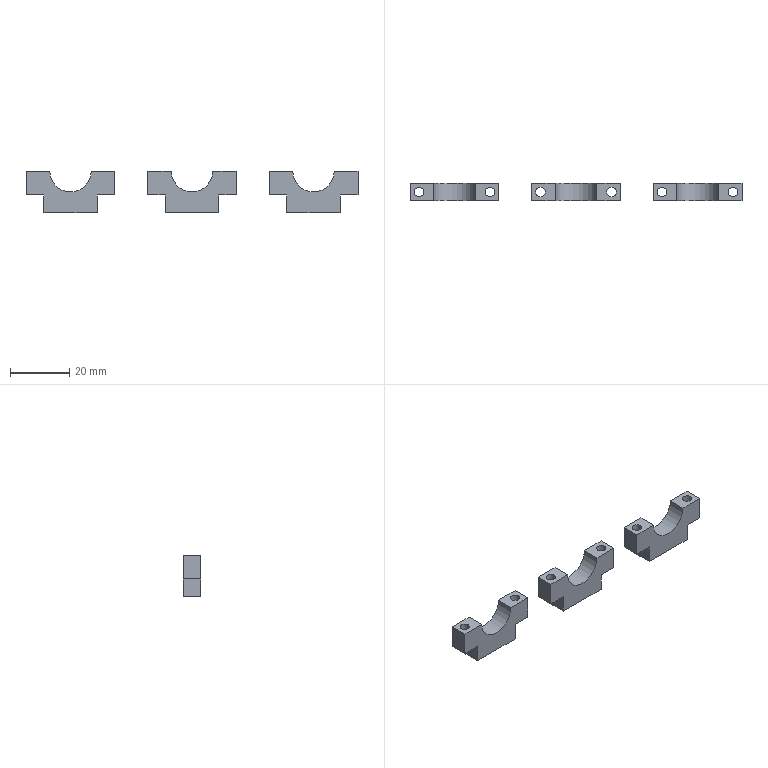CAM job | NX | 3+2 milling | part box 112 x 6 x 14 mm | stock box 117 x 10 x 15 mm
Tools:
number,name,description,diameter,corner_radius,flute_length,length,flutes
9,D10,平底铣刀-粗,10.0,0.0,35.0,75.0,2
17,D2-J,平底铣刀-精,2.0,0.0,50.0,75.0,2
7,D6-J,平底铣刀-精,6.0,0.0,25.0,75.0,2
10,D10-J,平底铣刀-精,10.0,0.0,35.0,75.0,2
1,D80R0.8飞刀,圆鼻刀-粗,80.0,0.8,50.0,75.0,2
2,D6倒角刀,倒角刀,6.0,0.0,3.0,25.0,2
Operations:
program,operation,operation_type,tool,method,geometry_group,spindle_rpm,surface_speed,feed_per_tooth,feed_cut,feed_plunge,cut_length_mm,path_length_mm,cut_time_min,machine_time_min
B,面铣自动飞面开粗_COPY,FaceMilling,D10,分层开粗-切深K-步距G,W-B,4500.0,890.615,0.3333,3000.0,100.0,2831.184,3823.767,0.9437,1.043
B,面铣自动飞面精光_COPY,FaceMilling,D10-J,侧刃精光-切深K-步距G,W-B,4500.0,890.615,0.1111,1000.0,100.0,406.0,502.0,0.406,0.4156
B,平面去毛刺6X45L_COPY,SurfaceContour,D6倒角刀,爬面_倒角-切深0-步距G,W-B,6500.0,122.519,0.1154,1500.0,100.0,315.202,534.628,0.2101,0.2321
A,顶面,FaceMilling,D80R0.8飞刀,侧刃精光-切深K-步距G,W-A,4500.0,1385.0,0.1667,1500.0,100.0,206.0,302.0,0.1373,0.1469
A,外形粗_2,VolumeBased25DMillingOperation,D10,METHOD,W-A,8000.0,251.327,0.375,6000.0,80.0,3714.282,4108.782,0.619,0.6585
A,等高光顺清角D2参考6_COPY,ZLevelMilling,D2-J,分层精光-切深K-步距G,W-A,8000.0,50.266,0.0938,1500.0,100.0,2413.35,3134.754,1.609,1.681
A,仅选体,SurfaceContour,D6倒角刀,METHOD,W-A,8000.0,150.796,0.1875,3000.0,100.0,336.57,706.972,0.1122,0.1492
A,外形半精_2,VolumeBased25DMillingOperation,D6-J,METHOD,W-A,9000.0,169.646,0.0667,1200.0,100.0,351.545,761.511,0.293,0.334